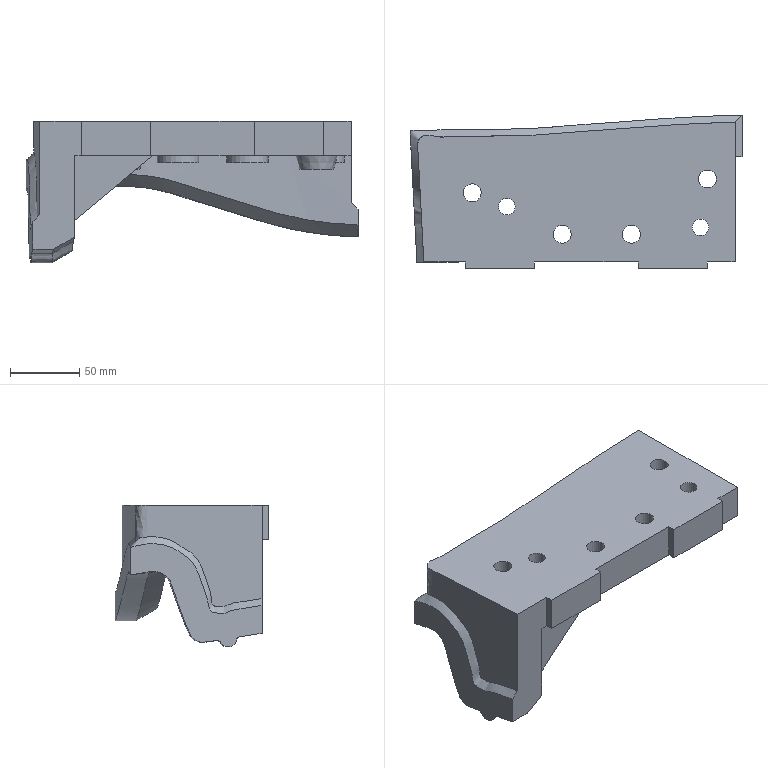Part | NX | features solid 2 | 1 solid | 48 faces | box 240 x 111.264 x 102.644 mm | volume 922383 mm3 | plane 27 | cylinder 13 | spline 6 | cone 2 | commonest cylinder face diameters 13 x6 30 x5 12 x2